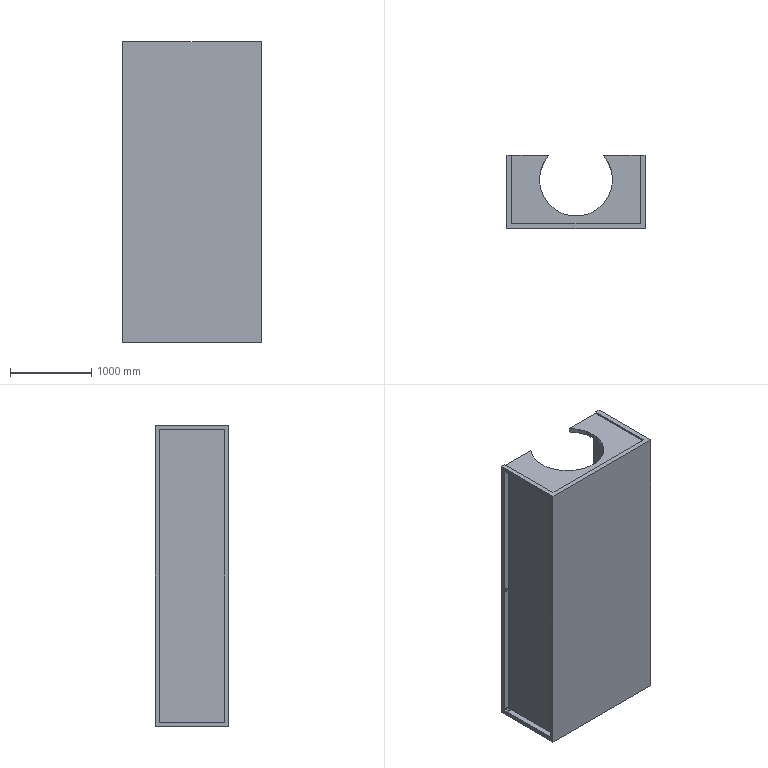Part | SolidWorks | features ICE 37, Extrusion 1 | 1 solid | 57 faces | box 1700 x 900 x 3700 mm | volume 580031915 mm3 | plane 37 | cylinder 20 | commonest cylinder face diameters 40 x12 900 x6 50 x2